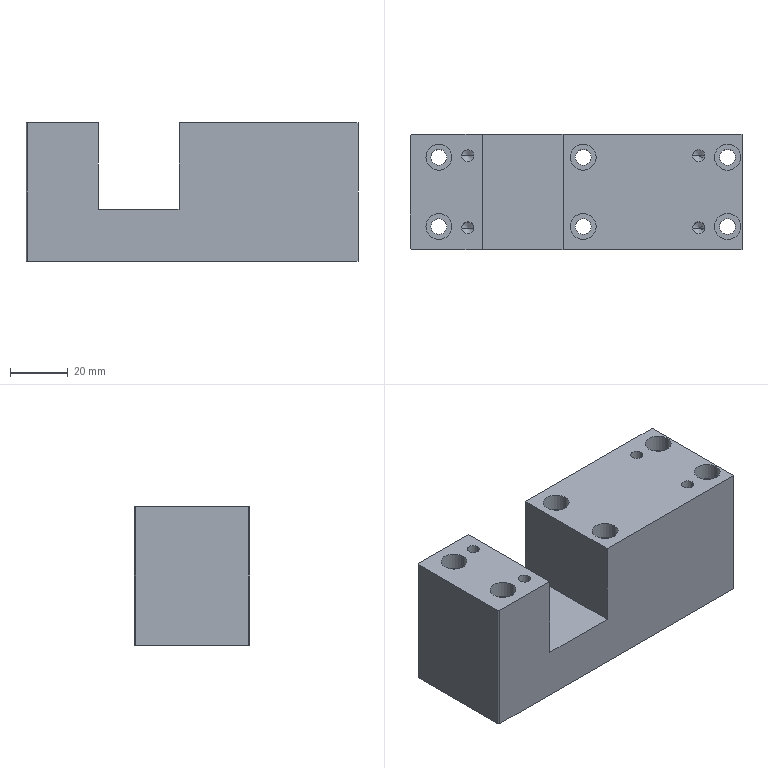Part | STEP file | spacer block 4 | 1 solid | 58 faces | box 115 x 40 x 48 mm | volume 178112 mm3 | cylinder 32 | plane 18 | cone 8 | commonest cylinder face diameters 5.5 x12 9 x12 4.2 x8